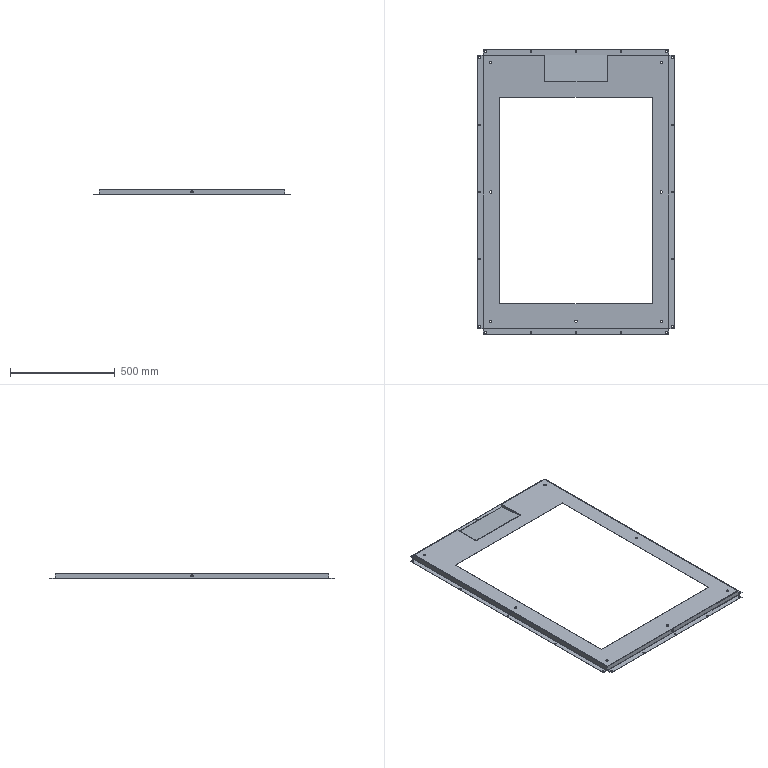Part | SolidWorks | 2 solids | 214 faces | box 939 x 1359 x 25.12 mm | volume 653415 mm3 | plane 110 | cylinder 92 | spline 12 | commonest cylinder face diameters 7 x50 11 x14 0.4 x11 2.4 x11 10 x6